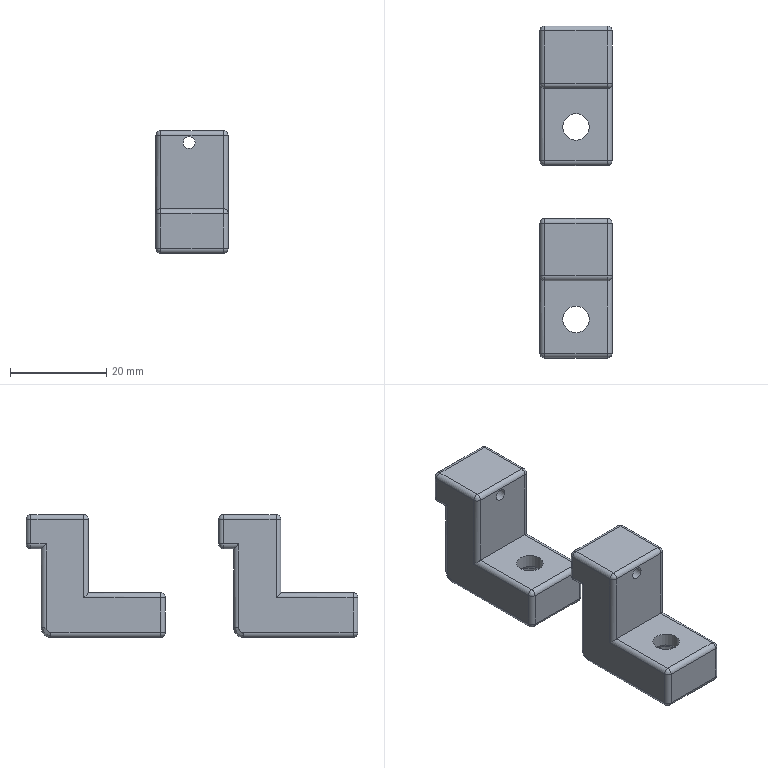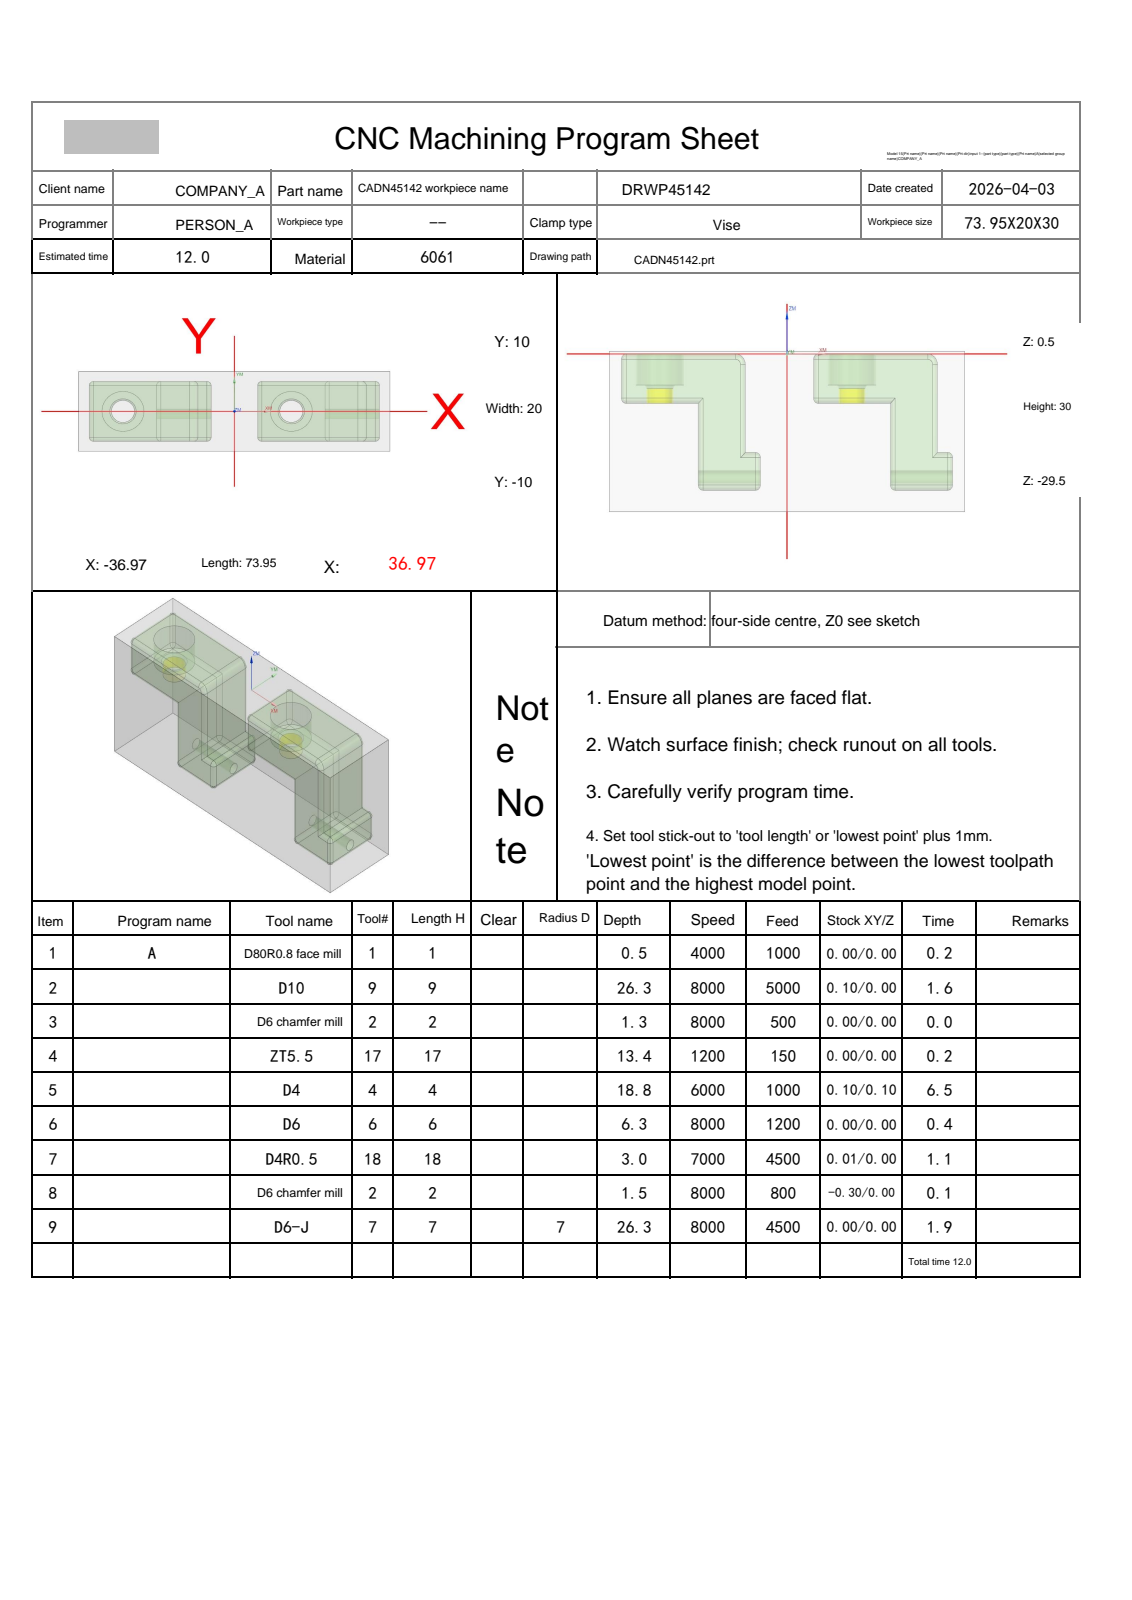NC program | NX | posted by the shop | part box 15 x 68.95 x 25.5 mm
Lines 3215 to 4664 of 6074:
N6 T06 M06
(D6  D=6. R=0. H=06 ce=0.10 di=0.00)
G00 G90 G54 X-26.475 Y0.0 M03 S8000
G43 H06 Z20.
M08
Z.5
G03 X-25.525 Y.95 I0.0 J.95 F1200.
X-26.475 Y1.9 I-.95 J0.0
X-26.475 Y1.9 Z0.0 I0.0 J-1.9
X-26.475 Y1.9 Z-.5 I0.0 J-1.9
X-26.475 Y1.9 Z-1. I0.0 J-1.9
X-26.475 Y1.9 Z-1.5 I0.0 J-1.9
X-26.475 Y1.9 Z-2. I0.0 J-1.9
X-26.475 Y1.9 Z-2.5 I0.0 J-1.9
X-26.475 Y1.9 Z-3. I0.0 J-1.9
X-26.475 Y1.9 Z-3.5 I0.0 J-1.9
X-26.475 Y1.9 Z-4. I0.0 J-1.9
X-26.475 Y1.9 Z-4.5 I0.0 J-1.9
X-26.475 Y1.9 Z-5. I0.0 J-1.9
X-26.475 Y1.9 Z-5.5 I0.0 J-1.9
X-25.358 Y-1.537 Z-5.8 I0.0 J-1.9
X-24.575 Y0.0 I-1.117 J1.537
X-26.475 Y1.9 I-1.9 J0.0
X-28.375 Y0.0 I0.0 J-1.9
X-26.475 Y-1.9 I1.9 J0.0
X-25.358 Y-1.537 I0.0 J1.9
X-24.966 Y-.769 I-.558 J.769
X-25.916 Y.181 I-.95 J0.0
X-26.475 Y0.0 I0.0 J-.95
G00 Z20.
X13.525
Z.5
G03 X14.475 Y.95 I0.0 J.95
X13.525 Y1.9 I-.95 J0.0
X13.525 Y1.9 Z0.0 I0.0 J-1.9
X13.525 Y1.9 Z-.5 I0.0 J-1.9
X13.525 Y1.9 Z-1. I0.0 J-1.9
X13.525 Y1.9 Z-1.5 I0.0 J-1.9
X13.525 Y1.9 Z-2. I0.0 J-1.9
X13.525 Y1.9 Z-2.5 I0.0 J-1.9
X13.525 Y1.9 Z-3. I0.0 J-1.9
X13.525 Y1.9 Z-3.5 I0.0 J-1.9
X13.525 Y1.9 Z-4. I0.0 J-1.9
X13.525 Y1.9 Z-4.5 I0.0 J-1.9
X13.525 Y1.9 Z-5. I0.0 J-1.9
X13.525 Y1.9 Z-5.5 I0.0 J-1.9
X14.642 Y-1.537 Z-5.8 I0.0 J-1.9
X15.425 Y0.0 I-1.117 J1.537
X13.525 Y1.9 I-1.9 J0.0
X11.625 Y0.0 I0.0 J-1.9
X13.525 Y-1.9 I1.9 J0.0
X14.642 Y-1.537 I0.0 J1.9
X15.034 Y-.769 I-.558 J.769
X14.084 Y.181 I-.95 J0.0
X13.525 Y0.0 I0.0 J-.95
G00 Z20.
G00 G90 X-26.475 Y0.0 M03 S8000
Z20.
Z0.0
G41 D06
G01 X-26.279 Y.039 F500.
G03 X-25.485 Y1.01 I-.196 J.97
X-26.475 Y2. I-.99 J0.0
X-26.475 Y2. Z-5. I0.0 J-2.
X-28.163 Y1.071 Z-5.8 I0.0 J-2.
X-28.475 Y0.0 I1.689 J-1.072
X-26.475 Y-2. I2. J0.0
X-24.475 Y0.0 I0.0 J2.
X-26.475 Y2. I-2. J0.0
X-28.163 Y1.071 I0.0 J-2.
X-28.318 Y.541 I.836 J-.53
X-27.328 Y-.449 I.99 J0.0
X-26.613 Y-.145 I0.0 J.99
G01 G40 X-26.475 Y0.0
G00 Z20.
X13.525
Z0.0
G41 D06
G01 X13.721 Y.039
G03 X14.515 Y1.01 I-.196 J.97
X13.525 Y2. I-.99 J0.0
X13.525 Y2. Z-5. I0.0 J-2.
X11.837 Y1.071 Z-5.8 I0.0 J-2.
X11.525 Y0.0 I1.689 J-1.072
X13.525 Y-2. I2. J0.0
X15.525 Y0.0 I0.0 J2.
X13.525 Y2. I-2. J0.0
X11.837 Y1.071 I0.0 J-2.
X11.682 Y.541 I.836 J-.53
X12.672 Y-.449 I.99 J0.0
X13.387 Y-.145 I0.0 J.99
G01 G40 X13.525 Y0.0
G00 Z20.
G91 G28 Z0.0
M05
M09
G91 G28 Z0.0
M01
N7 T18 M06
(D4R0.5  D=4. R=0.5 H=18 ce=0.01 di=0.00)
G00 G90 G54 X33.75 Y-7.915 M03 S7000
G43 H18 Z10.5
M08
Z.488
G01 Z-.012 F4500.
X30.426 Y-8.129
X29.326 Y-8.2
X6.525
G02 X4.825 Y-6.5 I0.0 J1.7
G01 Y6.5
G02 X6.525 Y8.2 I1.7 J0.0
G01 X29.325
X30.425 Y8.129
Y8.224 Z-.021
Y8.27 Z-.03
X29.325 Y8.309
X6.525
G03 X4.716 Y6.5 I0.0 J-1.809
G01 Y-6.5
G03 X6.525 Y-8.309 I1.809 J0.0
G01 X29.326
X30.426 Y-8.271
Y-8.345 Z-.042
X30.427 Y-8.391 Z-.054
X29.326 Y-8.408
X6.525
G02 X4.617 Y-6.5 I0.0 J1.909
G01 Y6.5
G02 X6.525 Y8.408 I1.909 J0.0
G01 X29.325
X30.425 Y8.387
X30.325 Y8.479 Z-.084
X29.325 Y8.504
X6.525
G03 X4.521 Y6.5 I0.0 J-2.004
G01 Y-6.5
G03 X6.525 Y-8.504 I2.004 J0.0
G01 X29.326
X30.426 Y-8.48
Y-8.528 Z-.102
Y-8.576 Z-.119
X29.326 Y-8.597
X6.525
G02 X4.429 Y-6.5 I0.0 J2.097
G01 Y6.5
G02 X6.525 Y8.597 I2.097 J0.0
G01 X29.325
X30.426 Y8.573
Y8.621 Z-.14
Y8.667 Z-.161
X29.325 Y8.687
X6.525
G03 X4.338 Y6.5 I0.0 J-2.187
G01 Y-6.5
G03 X6.525 Y-8.687 I2.187 J0.0
G01 X29.326
X30.437 Y-8.667
X30.433 Y-8.713 Z-.185
X30.429 Y-8.762 Z-.209
X29.326 Y-8.774
X6.525
G02 X4.251 Y-6.5 I0.0 J2.274
G01 Y6.5
G02 X6.525 Y8.774 I2.274 J0.0
G01 X29.325
X30.426 Y8.761
Y8.802 Z-.236
Y8.838 Z-.263
X29.325 Y8.858
X6.525
G03 X4.167 Y6.5 I0.0 J-2.359
G01 Y-6.5
G03 X6.525 Y-8.858 I2.359 J0.0
G01 X29.326
X30.426 Y-8.846
Y-8.885 Z-.293
X30.427 Y-8.918 Z-.322
X29.326 Y-8.939
X6.525
G02 X4.087 Y-6.5 I0.0 J2.439
G01 Y6.5
G02 X6.525 Y8.939 I2.439 J0.0
G01 X29.325
X30.421 Y8.916
Y8.952 Z-.354
Y8.989 Z-.386
X29.325 Y9.014
X6.525
G03 X4.011 Y6.5 I0.0 J-2.515
G01 Y-6.5
G03 X6.525 Y-9.014 I2.515 J0.0
G01 X29.326
X30.427 Y-8.99
Y-9.026 Z-.421
X30.426 Y-9.063 Z-.455
G03 X30.169 Y-9.061 I-.257 J-13.991
X29.326 Y-9.086 I0.0 J-13.993
G01 X6.525
G02 X3.939 Y-6.5 I0.0 J2.586
G01 Y6.5
G02 X6.525 Y9.086 I2.586 J0.0
G01 X29.325
G03 X30.178 Y9.059 I.853 J13.444
X30.421 Y9.061 I0.0 J13.471
G01 X30.424 Y9.099 Z-.492
X30.426 Y9.13 Z-.529
G02 X30.148 Y9.127 I-.279 J12.986
X29.325 Y9.153 I0.0 J12.989
G01 X6.525
G03 X3.872 Y6.5 I0.0 J-2.653
G01 Y-6.5
G03 X6.525 Y-9.153 I2.653 J0.0
G01 X29.326
G02 X30.192 Y-9.129 I.866 J-15.495
X30.426 Y-9.131 I0.0 J-15.52
G01 X30.427 Y-9.165 Z-.568
Y-9.196 Z-.607
G03 X29.326 Y-9.215 I1.173 J-101.223
G01 X6.525
G02 X3.81 Y-6.5 I0.0 J2.715
G01 Y6.5
G02 X6.525 Y9.215 I2.715 J0.0
G01 X29.325
X30.426 Y9.2
Y9.23 Z-.648
Y9.262 Z-.689
X29.325 Y9.272
X6.525
G03 X3.753 Y6.5 I0.0 J-2.772
G01 Y-6.5
G03 X6.525 Y-9.272 I2.772 J0.0
G01 X29.326
G02 X30.246 Y-9.258 I.92 J-31.243
G01 X30.427 Y-9.259
X30.426 Y-9.291 Z-.732
Y-9.316 Z-.775
X29.326 Y-9.323
X6.525
G02 X3.702 Y-6.5 I0.0 J2.823
G01 Y6.5
G02 X6.525 Y9.323 I2.823 J0.0
G01 X29.325
X30.425 Y9.316
X30.426 Y9.337 Z-.82
Y9.358 Z-.864
X29.325 Y9.368
X6.525
G03 X3.657 Y6.5 I0.0 J-2.869
G01 Y-6.5
G03 X6.525 Y-9.368 I2.869 J0.0
G01 X29.326
X30.426 Y-9.358
Y-9.376 Z-.91
Y-9.397 Z-.956
X30.392
X29.326 Y-9.408
X6.525
G02 X3.617 Y-6.5 I0.0 J2.908
G01 Y6.5
G02 X6.525 Y9.408 I2.908 J0.0
G01 X29.325
X30.392 Y9.396
X30.426 Y9.397
Y9.414 Z-1.003
Y9.428 Z-1.051
X30.22 Y9.427
G02 X29.325 Y9.441 I0.0 J29.627
G01 X6.525
G03 X3.584 Y6.5 I0.0 J-2.941
G01 Y-6.5
G03 X6.525 Y-9.441 I2.941 J0.0
G01 X29.326
G02 X30.193 Y-9.427 I.867 J-27.33
G01 X30.427 Y-9.428
X30.424 Y-9.446 Z-1.099
X30.422 Y-9.458 Z-1.147
X29.326 Y-9.468
X6.525
G02 X3.557 Y-6.5 I0.0 J2.968
G01 Y6.5
G02 X6.525 Y9.468 I2.968 J0.0
G01 X29.325
X30.422 Y9.458
Y9.462 Z-1.191
Y9.477 Z-1.235
X29.325 Y9.486
X6.525
G03 X3.539 Y6.5 I0.0 J-2.986
G01 Y-6.5
G03 X6.525 Y-9.486 I2.986 J0.0
G01 X29.326
X30.422 Y-9.477
Y-9.484 Z-1.279
Y-9.49 Z-1.323
G03 X30.133 Y-9.488 I-.289 J-29.016
X29.326 Y-9.499 I0.0 J-29.017
G01 X6.525
G02 X3.526 Y-6.5 I0.0 J3.
G01 Y6.5
G02 X6.525 Y9.499 I3. J0.0
G01 X29.325
G03 X30.137 Y9.488 I.811 J29.996
X30.422 Y9.49 I0.0 J30.007
G01 Y9.494 Z-1.368
Y9.5 Z-1.412
X29.325 Y9.507
X6.525
G03 X3.518 Y6.5 I0.0 J-3.007
G01 Y-6.5
G03 X6.525 Y-9.507 I3.007 J0.0
G01 X29.326
X30.422 Y-9.5
Y-9.51 Z-1.5
X29.326
X6.525
X6.404 Y-9.507
G02 X3.517 Y-6.615 I.121 J3.008
G01 X3.516 Y-6.561
Y6.5
X3.517 Y6.615
G02 X6.404 Y9.507 I3.008 J-.115
G01 X6.525 Y9.51
X29.325
X30.422
G00 Z10.5
X-6.38 Y-8.25
Z.488
G01 Z-.012
X-9.574 Y-8.129
X-10.674 Y-8.2
X-33.475
G02 X-35.175 Y-6.5 I0.0 J1.7
G01 Y6.5
G02 X-33.475 Y8.2 I1.7 J0.0
G01 X-10.675
X-9.575 Y8.129
Y8.224 Z-.021
Y8.27 Z-.03
X-10.675 Y8.309
X-33.475
G03 X-35.284 Y6.5 I0.0 J-1.809
G01 Y-6.5
G03 X-33.475 Y-8.309 I1.809 J0.0
G01 X-10.674
X-9.574 Y-8.27
Y-8.345 Z-.042
Y-8.385 Z-.054
X-9.631 Y-8.375
X-10.659 Y-8.402
X-10.674 Y-8.408
X-33.475
G02 X-35.383 Y-6.5 I0.0 J1.909
G01 Y6.5
G02 X-33.475 Y8.408 I1.909 J0.0
G01 X-10.675
X-9.575 Y8.386
X-9.574 Y8.438 Z-.069
Y8.479 Z-.084
X-10.675 Y8.504
X-33.475
G03 X-35.479 Y6.5 I0.0 J-2.004
G01 Y-6.5
G03 X-33.475 Y-8.504 I2.004 J0.0
G01 X-10.674
X-9.574 Y-8.478
Y-8.529 Z-.102
X-9.573 Y-8.571 Z-.119
X-10.674 Y-8.597
X-33.475
G02 X-35.571 Y-6.5 I0.0 J2.097
G01 Y6.5
G02 X-33.475 Y8.597 I2.097 J0.0
G01 X-10.675
X-9.574 Y8.573
Y8.62 Z-.14
Y8.667 Z-.161
X-10.675 Y8.687
X-33.475
G03 X-35.662 Y6.5 I0.0 J-2.187
G01 Y-6.5
G03 X-33.475 Y-8.687 I2.187 J0.0
G01 X-10.674
X-9.57 Y-8.667
X-9.569 Y-8.713 Z-.185
X-9.567 Y-8.763 Z-.209
X-10.674 Y-8.774
X-33.475
G02 X-35.749 Y-6.5 I0.0 J2.274
G01 Y6.5
G02 X-33.475 Y8.774 I2.274 J0.0
G01 X-10.675
X-9.574 Y8.761
Y8.802 Z-.236
Y8.838 Z-.263
X-10.659 Y8.855
X-10.675 Y8.858
X-33.475
G03 X-35.833 Y6.5 I0.0 J-2.359
G01 Y-6.5
G03 X-33.475 Y-8.858 I2.359 J0.0
G01 X-10.674
X-9.574 Y-8.845
Y-8.88 Z-.293
Y-8.918 Z-.322
X-10.674 Y-8.939
X-33.475
G02 X-35.913 Y-6.5 I0.0 J2.439
G01 Y6.5
G02 X-33.475 Y8.939 I2.439 J0.0
G01 X-10.675
X-9.574 Y8.916
Y8.952 Z-.354
Y8.989 Z-.386
X-10.675 Y9.014
X-33.475
G03 X-35.989 Y6.5 I0.0 J-2.515
G01 Y-6.5
G03 X-33.475 Y-9.014 I2.515 J0.0
G01 X-10.674
X-9.574 Y-8.99
Y-9.029 Z-.421
X-9.575 Y-9.063 Z-.455
X-9.608 Y-9.061
X-10.659 Y-9.081
X-10.674 Y-9.086
X-33.475
G02 X-36.061 Y-6.5 I0.0 J2.586
G01 Y6.5
G02 X-33.475 Y9.086 I2.586 J0.0
G01 X-10.675
X-10.659 Y9.081
X-9.621 Y9.063
X-9.574 Y9.064
Y9.099 Z-.492
X-9.575 Y9.132 Z-.529
G02 X-9.872 Y9.128 I-.297 J13.112
X-10.675 Y9.153 I0.0 J13.115
G01 X-33.475
G03 X-36.128 Y6.5 I0.0 J-2.653
G01 Y-6.5
G03 X-33.475 Y-9.153 I2.653 J0.0
G01 X-10.674
X-10.659 Y-9.15
X-9.573 Y-9.129
Y-9.165 Z-.568
Y-9.198 Z-.607
X-10.659 Y-9.21
X-10.674 Y-9.215
X-33.475
G02 X-36.19 Y-6.5 I0.0 J2.715
G01 Y6.5
G02 X-33.475 Y9.215 I2.715 J0.0
G01 X-10.675
X-9.575 Y9.2
Y9.23 Z-.648
Y9.263 Z-.689
X-10.659 Y9.266
X-10.675 Y9.272
X-33.475
G03 X-36.247 Y6.5 I0.0 J-2.772
G01 Y-6.5
G03 X-33.475 Y-9.272 I2.772 J0.0
G01 X-10.674
X-10.659 Y-9.266
X-9.574 Y-9.261
Y-9.291 Z-.732
Y-9.316 Z-.775
X-10.674 Y-9.323
X-33.475
G02 X-36.298 Y-6.5 I0.0 J2.823
G01 Y6.5
G02 X-33.475 Y9.323 I2.823 J0.0
G01 X-10.675
X-9.575 Y9.316
Y9.337 Z-.82
X-9.574 Y9.358 Z-.864
X-10.675 Y9.368
X-33.475
G03 X-36.343 Y6.5 I0.0 J-2.869
G01 Y-6.5
G03 X-33.475 Y-9.368 I2.869 J0.0
G01 X-10.674
X-9.574 Y-9.358
Y-9.376 Z-.91
Y-9.396 Z-.956
X-10.674 Y-9.408
X-33.475
G02 X-36.383 Y-6.5 I0.0 J2.908
G01 Y6.5
G02 X-33.475 Y9.408 I2.908 J0.0
G01 X-10.675
X-9.574 Y9.396
Y9.413 Z-1.003
Y9.428 Z-1.051
X-10.659 Y9.438
X-10.675 Y9.441
X-33.475
G03 X-36.416 Y6.5 I0.0 J-2.941
G01 Y-6.5
G03 X-33.475 Y-9.441 I2.941 J0.0
G01 X-10.674
X-10.659 Y-9.438
X-9.573 Y-9.428
X-9.572 Y-9.446 Z-1.099
X-9.571 Y-9.458 Z-1.147
X-10.674 Y-9.468
X-33.475
G02 X-36.443 Y-6.5 I0.0 J2.968
G01 Y6.5
G02 X-33.475 Y9.468 I2.968 J0.0
G01 X-10.675
X-9.571 Y9.458
Y9.462 Z-1.191
Y9.477 Z-1.235
X-10.675 Y9.486
X-33.475
G03 X-36.461 Y6.5 I0.0 J-2.986
G01 Y-6.5
G03 X-33.475 Y-9.486 I2.986 J0.0
G01 X-10.674
X-9.571 Y-9.477
Y-9.484 Z-1.279
Y-9.49 Z-1.323
X-10.659 Y-9.498
X-10.674 Y-9.499
X-33.475
G02 X-36.474 Y-6.5 I0.0 J3.
G01 Y6.5
G02 X-33.475 Y9.499 I3. J0.0
G01 X-10.675
X-10.659 Y9.498
X-9.571 Y9.49
Y9.494 Z-1.368
Y9.5 Z-1.412
X-10.659 Y9.504
X-10.675 Y9.507
X-33.475
G03 X-36.482 Y6.5 I0.0 J-3.007
G01 Y-6.5
G03 X-33.475 Y-9.507 I3.007 J0.0
G01 X-10.674
X-10.659 Y-9.504
X-9.571 Y-9.5
Y-9.51 Z-1.5
X-33.475
X-33.59 Y-9.508
G02 X-36.483 Y-6.615 I.115 J3.008
G01 X-36.484 Y-6.5
Y6.5
X-36.483 Y6.615
G02 X-33.475 Y9.51 I3.008 J-.115
G01 X-10.675
X-9.571
G00 Z10.5
G00 G90 X27.61 Y8.973 M03 S7000
Z10.5
Z.491
G01 Z-.009 F4500.
Y8.949
G03 X28.214 Y8.173 I.8 J0.0
X28.788 Y8.102 I.575 J2.272
X29.084 Y8.121 I0.0 J2.343
G02 X29.304 Y8.134 I.22 J-1.733
X31.047 Y6.5 I0.0 J-1.746
G01 Y-6.48
G02 X29.334 Y-8.166 I-1.812 J.127
G01 X29.263 Y-8.116
X28.214 Y-8.173
Y-8.223 Z-.015
Y-8.262 Z-.021
X29.263 Y-8.222
X29.334 Y-8.252
G03 X31.162 Y-6.5 I-.057 J1.889
G01 Y6.5
G03 X29.274 Y8.254 I-1.888 J-.139
G01 X29.192 Y8.252
X29.051 Y8.222
X28.214 Y8.262
Y8.306 Z-.03
Y8.345 Z-.038
X29.562 Y8.326
X29.617 Y8.316
G02 X31.269 Y6.5 I-.321 J-1.951
G01 Y-6.5
G02 X29.334 Y-8.342 I-1.973 J.136
G01 X28.214 Y-8.345
Y-8.386 Z-.048
Y-8.424 Z-.058
X29.617 Y-8.381
X29.735 Y-8.36
G03 X31.372 Y-6.5 I-.344 J1.954
G01 Y6.5
G03 X29.461 Y8.386 I-1.971 J-.086
G01 X28.214 Y8.424
Y8.464 Z-.07
Y8.5 Z-.083
G02 X28.757 Y8.531 I.544 J-4.85
X30.067 Y8.352 I0.0 J-4.881
X31.472 Y6.502 I-.515 J-1.85
G01 X31.473 Y-6.502
G02 X30.068 Y-8.352 I-1.92 J0.0
X28.758 Y-8.531 I-1.31 J4.705
X28.214 Y-8.5 I0.0 J4.884
G01 Y-8.539 Z-.097
Y-8.575 Z-.111
G03 X28.762 Y-8.604 I.548 J5.132
X29.966 Y-8.462 I0.0 J5.161
X31.571 Y-6.5 I-.489 J2.038
G01 Y6.5
G03 X29.966 Y8.462 I-2.095 J-.076
X28.762 Y8.604 I-1.204 J-5.014
X28.214 Y8.575 I0.0 J-5.157
G01 Y8.613 Z-.127
Y8.648 Z-.143
X29.617 Y8.623
X29.901 Y8.568
G02 X31.668 Y6.5 I-.446 J-2.17
G01 Y-6.5
G02 X29.901 Y-8.568 I-2.213 J.102
G01 X29.617 Y-8.623
X28.214 Y-8.648
Y-8.685 Z-.16
Y-8.719 Z-.178
X29.617 Y-8.692
X29.833 Y-8.659
G03 X31.763 Y-6.5 I-.351 J2.256
G01 Y6.5
G03 X29.833 Y8.659 I-2.281 J-.098
G01 X29.617 Y8.692
X28.214 Y8.719
Y8.755 Z-.198
Y8.788 Z-.218
G02 X28.68 Y8.8 I.466 J-9.521
X29.773 Y8.737 I0.0 J-9.532
X31.856 Y6.5 I-.27 J-2.339
G01 Y-6.5
G02 X29.773 Y-8.737 I-2.353 J.103
X28.68 Y-8.8 I-1.093 J9.48
X28.214 Y-8.788 I0.0 J9.543
G01 Y-8.823 Z-.239
Y-8.855 Z-.261
G03 X28.678 Y-8.866 I.464 J9.729
X29.799 Y-8.801 I0.0 J9.741
X31.948 Y-6.5 I-.28 J2.414
G01 X31.947 Y6.5
G03 X29.799 Y8.801 I-2.428 J-.113
X28.678 Y8.866 I-1.121 J-9.667
X28.214 Y8.855 I0.0 J-9.732
G01 Y8.888 Z-.284
Y8.92 Z-.307
G02 X28.763 Y8.939 I.549 J-7.787
X29.888 Y8.858 I0.0 J-7.806
X31.915 Y7.197 I-.366 J-2.514
G01 X32.021 Y6.632
X32.037 Y6.5
Y-6.5
G02 X30.868 Y-8.489 I-2.443 J.098
X29.685 Y-8.89 I-1.484 J2.429
X28.749 Y-8.934 I-.936 J9.962
X28.214 Y-8.92 I0.0 J10.006
G01 Y-8.952 Z-.333
Y-8.982 Z-.358
G03 X28.743 Y-9. I.529 J7.765
X30.046 Y-8.89 I0.0 J7.784
X32.124 Y-6.5 I-.456 J2.495
G01 Y6.5
G03 X30.046 Y8.89 I-2.535 J-.105
X28.743 Y9. I-1.303 J-7.673
X28.214 Y8.982 I0.0 J-7.783
G01 Y9.013 Z-.384
Y9.042 Z-.411
G02 X28.757 Y9.052 I.543 J-14.026
X29.537 Y9.03 I0.0 J-14.036
X31.03 Y8.558 I-.175 J-3.148
X32.209 Y6.5 I-1.325 J-2.126
G01 Y-6.5
G02 X30.751 Y-8.717 I-2.534 J.078
X29.334 Y-9.04 I-1.462 J3.139
G01 X28.228
X28.214 Y-9.042
Y-9.071 Z-.44
Y-9.098 Z-.468
G03 X28.709 Y-9.107 I.495 J14.3
X29.617 Y-9.078 I0.0 J14.309
X31.034 Y-8.637 I-.217 J3.195
X32.292 Y-6.5 I-1.314 J2.212
G01 Y6.5
G03 X31.919 Y7.761 I-2.546 J-.068
X29.798 Y9.058 I-2.405 J-1.551
X28.735 Y9.111 I-1.063 J-10.631
X28.214 Y9.098 I0.0 J-10.684
G01 Y9.126 Z-.498
Y9.153 Z-.528
G02 X28.758 Y9.168 I.544 J-9.529
X29.901 Y9.099 I0.0 J-9.545
X31.884 Y7.962 I-.397 J-2.992
X32.372 Y6.5 I-2.25 J-1.564
G01 X32.373 Y-6.5
G02 X31.2 Y-8.608 I-2.607 J.07
X29.617 Y-9.132 I-1.784 J2.734
X28.746 Y-9.165 I-.871 J11.643
X28.214 Y-9.153 I0.0 J11.676
G01 Y-9.179 Z-.56
Y-9.203 Z-.591
X28.228 Y-9.202
X29.334
X29.347
G03 X31.318 Y-8.61 I0.0 J3.578
X32.451 Y-6.5 I-1.534 J2.183
G01 X32.45 Y6.5
G03 X31.318 Y8.61 I-2.668 J-.073
X29.346 Y9.202 I-1.971 J-2.986
G01 X29.334
X28.227
X28.214 Y9.203
Y9.228 Z-.625
Y9.251 Z-.658
X29.334
X29.338
G02 X31.034 Y8.849 I0.0 J-3.776
X32.526 Y6.5 I-1.207 J-2.414
G01 Y-6.5
G02 X31.034 Y-8.849 I-2.698 J.065
X29.339 Y-9.251 I-1.696 J3.376
G01 X29.334
X28.214
Y-9.274 Z-.692
Y-9.295 Z-.727
X29.334
X29.346
G03 X31.034 Y-8.915 I0.0 J3.936
X32.598 Y-6.5 I-1.184 J2.481
G01 Y6.5
G03 X31.318 Y8.753 I-2.716 J-.054
X29.617 Y9.281 I-1.873 J-3.031
X28.6 Y9.298 I-1.017 J-30.065
X28.214 Y9.295 I0.0 J-30.082
G01 Y9.316 Z-.763
Y9.336 Z-.799
G02 X28.761 Y9.349 I.547 J-11.927
X29.901 Y9.294 I0.0 J-11.94
X31.601 Y8.621 I-.348 J-3.364
X32.668 Y6.5 I-1.652 J-2.16
G01 Y-6.5
G02 X31.318 Y-8.817 I-2.74 J.045
X29.901 Y-9.294 I-1.801 J3.002
X28.761 Y-9.349 I-1.139 J11.897
X28.214 Y-9.336 I0.0 J11.951
G01 Y-9.355 Z-.837
Y-9.373 Z-.874
X28.228 Y-9.372
X29.334
G03 X30.775 Y-9.131 I-.021 J4.565
X31.698 Y-8.608 I-.9 J2.661
G01 X31.884 Y-8.456
G03 X32.735 Y-6.5 I-1.936 J2.005
G01 X32.734 Y6.5
G03 X32.411 Y7.761 I-2.856 J-.06
X30.751 Y9.14 I-2.605 J-1.447
X29.334 Y9.372 I-1.437 J-4.341
G01 X28.227
X28.214 Y9.373
Y9.39 Z-.913
Y9.406 Z-.951
X28.227 Y9.403
X29.334
X29.372
G02 X30.467 Y9.264 I0.0 J-4.385
G01 X30.751 Y9.187
G02 X31.884 Y8.525 I-1.007 J-3.027
X32.798 Y6.5 I-1.859 J-2.058
G01 Y-6.5
G02 X31.884 Y-8.526 I-2.773 J.032
X30.751 Y-9.187 I-2.14 J2.365
G01 X30.467 Y-9.264
G02 X29.372 Y-9.403 I-1.095 J4.246
G01 X29.334
X28.228
X28.214 Y-9.406
Y-9.421 Z-.991
Y-9.435 Z-1.031
G03 X28.727 Y-9.443 I.513 J16.619
X29.901 Y-9.401 I0.0 J16.627
X31.488 Y-8.89 I-.312 J3.69
X32.859 Y-6.5 I-1.479 J2.437
G01 Y6.5
G03 X31.487 Y8.89 I-2.85 J-.047
X29.901 Y9.401 I-1.899 J-3.179
X28.727 Y9.443 I-1.174 J-16.57
X28.214 Y9.435 I0.0 J-16.612
G01 X28.216 Y9.448 Z-1.072
X28.218 Y9.459 Z-1.114
G02 X28.771 Y9.47 I.552 J-14.81
X29.901 Y9.426 I0.0 J-14.821
X31.601 Y8.871 I-.243 J-3.624
X32.916 Y6.5 I-1.559 J-2.414
G01 Y-6.5
G02 X31.601 Y-8.871 I-2.873 J.043
X29.901 Y-9.426 I-1.943 J3.068
X28.771 Y-9.47 I-1.13 J14.793
X28.218 Y-9.459 I0.0 J14.836
G01 Y-9.47 Z-1.156
Y-9.479 Z-1.198
X29.334 Y-9.477
X29.359
G03 X30.467 Y-9.371 I0.0 J5.888
X31.884 Y-8.72 I-.666 J3.313
X32.97 Y-6.5 I-1.806 J2.259
G01 Y6.5
G03 X32.878 Y7.197 I-4.117 J-.185
X31.034 Y9.202 I-2.865 J-.784
X29.617 Y9.471 I-1.51 J-4.089
G01 X28.218 Y9.479
Y9.487 Z-1.241
Y9.494 Z-1.284
G02 X29.617 Y9.486 I-.232 J-162.856
X31.203 Y9.172 I-.032 J-4.322
X32.719 Y7.761 I-1.193 J-2.802
X33.02 Y6.5 I-2.787 J-1.332
G01 Y-6.5
G02 X31.884 Y-8.775 I-2.93 J.042
X30.196 Y-9.441 I-2.097 J2.84
X29.363 Y-9.49 I-.833 J7.145
G01 X28.236
X28.218 Y-9.494
Y-9.504 Z-1.373
X28.236 Y-9.499
G03 X28.757 Y-9.502 I.521 J41.295
X29.901 Y-9.486 I0.0 J41.298
X31.318 Y-9.155 I-.181 J3.972
X33.067 Y-6.5 I-1.21 J2.701
G01 Y6.5
G03 X31.318 Y9.155 I-2.959 J-.046
X29.901 Y9.486 I-1.598 J-3.64
X28.755 Y9.502 I-1.146 J-41.506
X28.236 Y9.499 I0.0 J-41.522
G01 X28.218 Y9.504
Y9.509 Z-1.463
G02 X28.761 Y9.515 I.543 J-27.928
X30.09 Y9.483 I0.0 J-27.934
X32.168 Y8.632 I-.16 J-3.351
X33.11 Y6.5 I-2.058 J-2.184
G01 X33.111 Y-6.5
G02 X32.168 Y-8.633 I-3.001 J.052
X30.075 Y-9.483 I-2.237 J2.503
X28.697 Y-9.513 I-1.378 J32.018
X28.218 Y-9.509 I0.0 J32.048
G01 Y-9.51 Z-1.555
X29.617
X29.999 Y-9.498
G03 X31.312 Y-9.215 I-.119 J3.744
X33.018 Y-7.349 I-1.138 J2.752
X33.15 Y-6.5 I-3.615 J1.
G01 Y6.5
G03 X33.018 Y7.349 I-3.761 J-.152
X31.312 Y9.215 I-2.844 J-.886
X30.001 Y9.498 I-1.431 J-3.46
G01 X29.617 Y9.51
X28.218
Z-1.648
X29.617
X29.901 Y9.508
X29.923
G02 X31.318 Y9.241 I0.0 J-3.769
X33.186 Y6.5 I-1.122 J-2.772
G01 Y-6.5
G02 X31.318 Y-9.241 I-2.991 J.031
X29.922 Y-9.509 I-1.395 J3.505
G01 X29.901
X29.617 Y-9.51
X28.218
Z-1.743
X29.901
X30.184 Y-9.502
G03 X31.884 Y-8.967 I-.109 J3.317
X33.218 Y-6.5 I-1.662 J2.493
G01 Y6.5
G03 X31.884 Y8.967 I-2.996 J-.026
X30.184 Y9.502 I-1.81 J-2.783
G01 X29.901 Y9.51
X28.218
Z-1.839
X29.901
X30.184 Y9.505
G02 X32.363 Y8.608 I-.043 J-3.2
X33.246 Y6.5 I-2.149 J-2.139
G01 X33.247 Y-6.5
G02 X31.561 Y-9.172 I-2.999 J.023
G01 X31.318 Y-9.284
X31.034 Y-9.376
G02 X30.184 Y-9.505 I-.894 J3.014
G01 X29.901 Y-9.51
X28.218
Z-1.936
X30.184 Y-9.509
X30.361 Y-9.5
G03 X32.734 Y-8.201 I-.147 J3.085
X33.271 Y-6.5 I-2.563 J1.745
G01 Y6.5
G03 X32.734 Y8.2 I-3.102 J-.044
X30.361 Y9.5 I-2.52 J-1.786
G01 X30.184 Y9.509
X28.218 Y9.51
Z-2.034
X30.184
X30.361 Y9.503
G02 X32.858 Y8.043 I-.113 J-3.058
X33.292 Y6.5 I-2.658 J-1.58
G01 Y-6.5
G02 X30.751 Y-9.46 I-3.019 J.02
X30.184 Y-9.51 I-.629 J3.932
G01 X28.218
Z-2.133
X30.184
X30.361 Y-9.505
G03 X31.884 Y-9.051 I-.125 J3.198
X33.309 Y-6.5 I-1.617 J2.576
G01 X33.308 Y6.5
G03 X32.734 Y8.258 I-3.086 J-.035
X30.343 Y9.504 I-2.459 J-1.802
G01 X30.184 Y9.51
X28.218
Z-2.224
X30.184
X30.343 Y9.506
G02 X32.734 Y8.275 I-.055 J-3.045
X33.31 Y6.632 I-2.44 J-1.778
G01 X33.313 Y6.566
X33.32 Y6.5
X33.321 Y-6.5
X33.315 Y-6.516
X33.311 Y-6.632
G02 X31.671 Y-9.172 I-2.984 J.127
G01 X31.601 Y-9.208
G02 X30.343 Y-9.506 I-1.319 J2.763
G01 X30.184 Y-9.51
X28.218
Z-2.316
X30.361 Y-9.509
X30.467 Y-9.503
G03 X33.301 Y-6.866 I-.158 J3.011
G01 X33.329 Y-6.5
Y6.5
X33.322 Y6.566
X33.301 Y6.863
G03 X30.467 Y9.503 I-2.992 J-.371
G01 X30.361 Y9.509
X28.218 Y9.51
Z-2.408
X30.343
G02 X33.334 Y6.5 I-.032 J-3.022
G01 Y-6.5
G02 X30.343 Y-9.51 I-3.022 J.012
G01 X28.218
Z-2.5
X30.343
G03 X33.336 Y-6.5 I-.019 J3.011
G01 Y-.141
X33.335 Y6.49
Y6.498
G03 X30.343 Y9.51 I-3.011 J0.0
G01 X28.218
G00 Z10.5
X-12.39 Y8.973
Z.491
G01 Z-.009
Y8.949
G03 X-11.786 Y8.173 I.8 J0.0
X-11.212 Y8.102 I.575 J2.272
X-10.916 Y8.121 I0.0 J2.343
G02 X-10.696 Y8.134 I.22 J-1.733
X-8.953 Y6.5 I0.0 J-1.746
G01 Y-6.48
G02 X-10.666 Y-8.166 I-1.812 J.127
G01 X-10.737 Y-8.116
X-11.786 Y-8.173
Y-8.223 Z-.015
Y-8.262 Z-.021
X-10.737 Y-8.222
X-10.666 Y-8.252
G03 X-8.838 Y-6.5 I-.057 J1.889
G01 Y6.5
G03 X-10.726 Y8.254 I-1.888 J-.139
G01 X-10.808 Y8.252
X-10.949 Y8.222
X-11.786 Y8.262
Y8.306 Z-.03
Y8.345 Z-.038
X-10.438 Y8.326
X-10.383 Y8.316
G02 X-8.731 Y6.5 I-.321 J-1.951
G01 Y-6.5
G02 X-10.666 Y-8.342 I-1.973 J.136
G01 X-11.786 Y-8.345
Y-8.386 Z-.048
Y-8.424 Z-.058
X-10.383 Y-8.381
X-10.265 Y-8.36
G03 X-8.628 Y-6.5 I-.344 J1.954
G01 Y6.5
G03 X-10.539 Y8.386 I-1.971 J-.086
G01 X-11.786 Y8.424
Y8.464 Z-.07
Y8.5 Z-.083
G02 X-11.243 Y8.531 I.544 J-4.85
X-9.933 Y8.352 I0.0 J-4.881
X-8.528 Y6.502 I-.515 J-1.85
G01 X-8.527 Y-6.502
G02 X-9.932 Y-8.352 I-1.92 J0.0
X-11.243 Y-8.531 I-1.31 J4.705
X-11.786 Y-8.5 I0.0 J4.884
G01 Y-8.539 Z-.097
Y-8.575 Z-.111
G03 X-11.238 Y-8.604 I.548 J5.132
X-10.034 Y-8.462 I0.0 J5.161
X-8.429 Y-6.5 I-.489 J2.038
G01 Y6.5
G03 X-10.034 Y8.462 I-2.095 J-.076
X-11.238 Y8.604 I-1.204 J-5.014
X-11.786 Y8.575 I0.0 J-5.157
G01 Y8.613 Z-.127
Y8.648 Z-.143
X-10.383 Y8.623
X-10.099 Y8.568
G02 X-8.332 Y6.5 I-.446 J-2.17
G01 Y-6.5
G02 X-10.099 Y-8.568 I-2.213 J.102
G01 X-10.383 Y-8.623
X-11.786 Y-8.648
Y-8.685 Z-.16
Y-8.719 Z-.178
X-10.383 Y-8.692
X-10.167 Y-8.659
G03 X-8.237 Y-6.5 I-.351 J2.256
G01 Y6.5
G03 X-10.167 Y8.659 I-2.281 J-.098
G01 X-10.383 Y8.692
X-11.786 Y8.719
Y8.755 Z-.198
Y8.788 Z-.218
G02 X-11.32 Y8.8 I.466 J-9.521
X-10.227 Y8.737 I0.0 J-9.532
X-8.144 Y6.5 I-.27 J-2.339
G01 Y-6.5
G02 X-10.227 Y-8.737 I-2.353 J.103
X-11.32 Y-8.8 I-1.093 J9.48
X-11.786 Y-8.788 I0.0 J9.543
G01 Y-8.823 Z-.239
Y-8.855 Z-.261
G03 X-11.322 Y-8.866 I.464 J9.729
X-10.201 Y-8.801 I0.0 J9.741
X-8.052 Y-6.5 I-.28 J2.414
G01 X-8.053 Y6.5
G03 X-10.201 Y8.801 I-2.428 J-.113
X-11.322 Y8.866 I-1.121 J-9.667
X-11.786 Y8.855 I0.0 J-9.732
G01 Y8.888 Z-.284
Y8.92 Z-.307
G02 X-11.237 Y8.939 I.549 J-7.787
X-10.112 Y8.858 I0.0 J-7.806
X-8.085 Y7.197 I-.366 J-2.514
G01 X-7.979 Y6.632
X-7.963 Y6.5
Y-6.5
G02 X-9.132 Y-8.489 I-2.443 J.098
X-10.315 Y-8.89 I-1.484 J2.429
X-11.251 Y-8.934 I-.936 J9.962
X-11.786 Y-8.92 I0.0 J10.006
G01 Y-8.952 Z-.333
Y-8.982 Z-.358
G03 X-11.257 Y-9. I.529 J7.765
X-9.954 Y-8.89 I0.0 J7.784
X-7.876 Y-6.5 I-.456 J2.495
G01 Y6.5
G03 X-9.954 Y8.89 I-2.535 J-.105
X-11.257 Y9. I-1.303 J-7.673
X-11.786 Y8.982 I0.0 J-7.783
G01 Y9.013 Z-.384
Y9.042 Z-.411
G02 X-11.243 Y9.052 I.543 J-14.026
X-10.463 Y9.03 I0.0 J-14.036
X-8.97 Y8.558 I-.175 J-3.148
X-7.791 Y6.5 I-1.325 J-2.126
G01 Y-6.5
G02 X-9.249 Y-8.717 I-2.534 J.078
X-10.666 Y-9.04 I-1.462 J3.139
G01 X-11.772
X-11.786 Y-9.042
Y-9.071 Z-.44
Y-9.098 Z-.468
G03 X-11.291 Y-9.107 I.495 J14.3
X-10.383 Y-9.078 I0.0 J14.309
X-8.966 Y-8.637 I-.217 J3.195
X-7.708 Y-6.5 I-1.314 J2.212
G01 Y6.5
G03 X-8.081 Y7.761 I-2.546 J-.068
X-10.202 Y9.058 I-2.405 J-1.551
X-11.265 Y9.111 I-1.063 J-10.631
X-11.786 Y9.098 I0.0 J-10.684
G01 Y9.126 Z-.498
Y9.153 Z-.528
G02 X-11.242 Y9.168 I.544 J-9.529
X-10.099 Y9.099 I0.0 J-9.545
X-8.116 Y7.962 I-.397 J-2.992
X-7.628 Y6.5 I-2.25 J-1.564
G01 X-7.627 Y-6.5
G02 X-8.8 Y-8.608 I-2.607 J.07
X-10.383 Y-9.132 I-1.784 J2.734
X-11.254 Y-9.165 I-.871 J11.643
X-11.786 Y-9.153 I0.0 J11.676
G01 Y-9.179 Z-.56
Y-9.203 Z-.591
X-11.772 Y-9.202
X-10.666
X-10.653
G03 X-8.682 Y-8.61 I0.0 J3.578
X-7.549 Y-6.5 I-1.534 J2.183
G01 X-7.55 Y6.5
G03 X-8.682 Y8.61 I-2.668 J-.073
X-10.654 Y9.202 I-1.971 J-2.986
G01 X-10.666
X-11.773
X-11.786 Y9.203
Y9.228 Z-.625
Y9.251 Z-.658
X-10.666
X-10.662
G02 X-8.966 Y8.849 I0.0 J-3.776
X-7.474 Y6.5 I-1.207 J-2.414
G01 Y-6.5
G02 X-8.966 Y-8.849 I-2.698 J.065
X-10.661 Y-9.251 I-1.696 J3.376
G01 X-10.666
X-11.786
Y-9.274 Z-.692
Y-9.295 Z-.727
X-10.666
X-10.654
G03 X-8.966 Y-8.915 I0.0 J3.936
X-7.402 Y-6.5 I-1.184 J2.481
G01 Y6.5
G03 X-8.682 Y8.753 I-2.716 J-.054
X-10.383 Y9.281 I-1.873 J-3.031
X-11.4 Y9.298 I-1.017 J-30.065
X-11.786 Y9.295 I0.0 J-30.082
G01 Y9.316 Z-.763
Y9.336 Z-.799
G02 X-11.239 Y9.349 I.547 J-11.927
X-10.099 Y9.294 I0.0 J-11.94
X-8.399 Y8.621 I-.348 J-3.364
X-7.332 Y6.5 I-1.652 J-2.16
G01 Y-6.5
G02 X-8.682 Y-8.817 I-2.74 J.045
X-10.099 Y-9.294 I-1.801 J3.002
X-11.239 Y-9.349 I-1.139 J11.897
X-11.786 Y-9.336 I0.0 J11.951
G01 Y-9.355 Z-.837
Y-9.373 Z-.874
X-11.772 Y-9.372
X-10.666
G03 X-9.225 Y-9.131 I-.021 J4.565
X-8.302 Y-8.608 I-.9 J2.661
G01 X-8.116 Y-8.456
G03 X-7.265 Y-6.5 I-1.936 J2.005
G01 X-7.266 Y6.5
G03 X-7.589 Y7.761 I-2.856 J-.06
X-9.249 Y9.14 I-2.605 J-1.447
X-10.666 Y9.372 I-1.437 J-4.341
G01 X-11.773
X-11.786 Y9.373
Y9.39 Z-.913
Y9.406 Z-.951
X-11.773 Y9.403
X-10.666
X-10.628
G02 X-9.533 Y9.264 I0.0 J-4.385
G01 X-9.249 Y9.187
G02 X-8.116 Y8.525 I-1.007 J-3.027
X-7.202 Y6.5 I-1.859 J-2.058
G01 Y-6.5
G02 X-8.116 Y-8.526 I-2.773 J.032
X-9.249 Y-9.187 I-2.14 J2.365
G01 X-9.533 Y-9.264
G02 X-10.628 Y-9.403 I-1.095 J4.246
G01 X-10.666
X-11.772
X-11.786 Y-9.406
Y-9.421 Z-.991
Y-9.435 Z-1.031
G03 X-11.273 Y-9.443 I.513 J16.619
X-10.099 Y-9.401 I0.0 J16.627
X-8.512 Y-8.89 I-.312 J3.69
X-7.141 Y-6.5 I-1.479 J2.437
G01 Y6.5
G03 X-8.513 Y8.89 I-2.85 J-.047
X-10.099 Y9.401 I-1.899 J-3.179
X-11.273 Y9.443 I-1.174 J-16.57
X-11.786 Y9.435 I0.0 J-16.612
G01 X-11.784 Y9.448 Z-1.072
X-11.782 Y9.459 Z-1.114
G02 X-11.229 Y9.47 I.552 J-14.81
X-10.099 Y9.426 I0.0 J-14.821
X-8.399 Y8.871 I-.243 J-3.624
X-7.084 Y6.5 I-1.559 J-2.414
G01 Y-6.5
G02 X-8.399 Y-8.871 I-2.873 J.043
X-10.099 Y-9.426 I-1.943 J3.068
X-11.229 Y-9.47 I-1.13 J14.793
X-11.782 Y-9.459 I0.0 J14.836
G01 Y-9.47 Z-1.156
Y-9.479 Z-1.198
X-10.666 Y-9.477
X-10.641
G03 X-9.533 Y-9.371 I0.0 J5.888
X-8.116 Y-8.72 I-.666 J3.313
X-7.03 Y-6.5 I-1.806 J2.259
G01 Y6.5
G03 X-7.122 Y7.197 I-4.117 J-.185
X-8.966 Y9.202 I-2.865 J-.784
X-10.383 Y9.471 I-1.51 J-4.089
G01 X-11.782 Y9.479
Y9.487 Z-1.241
Y9.494 Z-1.284
G02 X-10.383 Y9.486 I-.232 J-162.856
X-8.797 Y9.172 I-.032 J-4.322
X-7.281 Y7.761 I-1.193 J-2.802
X-6.98 Y6.5 I-2.787 J-1.332
G01 Y-6.5
G02 X-8.116 Y-8.775 I-2.93 J.042
X-9.804 Y-9.441 I-2.097 J2.84
X-10.637 Y-9.49 I-.833 J7.145
G01 X-11.764
X-11.782 Y-9.494
Y-9.504 Z-1.373
X-11.764 Y-9.499
G03 X-11.243 Y-9.502 I.521 J41.294
X-10.099 Y-9.486 I0.0 J41.298
X-8.682 Y-9.155 I-.181 J3.972
X-6.933 Y-6.5 I-1.21 J2.701
G01 Y6.5
G03 X-8.682 Y9.155 I-2.959 J-.046
X-10.099 Y9.486 I-1.598 J-3.64
X-11.245 Y9.502 I-1.146 J-41.506
X-11.764 Y9.499 I0.0 J-41.522
G01 X-11.782 Y9.504
Y9.509 Z-1.463
G02 X-11.239 Y9.515 I.543 J-27.928
X-9.91 Y9.483 I0.0 J-27.934
X-7.832 Y8.632 I-.16 J-3.351
X-6.89 Y6.5 I-2.058 J-2.184
G01 X-6.889 Y-6.5
G02 X-7.832 Y-8.633 I-3.001 J.052
X-9.925 Y-9.483 I-2.237 J2.503
X-11.303 Y-9.513 I-1.378 J32.017
X-11.782 Y-9.509 I0.0 J32.046
G01 X-11.773 Y-9.51 Z-1.555
X-10.383
X-10.001 Y-9.498
G03 X-8.688 Y-9.215 I-.119 J3.744
X-6.982 Y-7.349 I-1.138 J2.752
X-6.85 Y-6.5 I-3.615 J1.
G01 Y6.5
G03 X-6.982 Y7.349 I-3.761 J-.152
X-8.688 Y9.215 I-2.844 J-.886
X-9.999 Y9.498 I-1.431 J-3.46
G01 X-10.383 Y9.51
X-11.782
Z-1.648
X-10.383
X-10.099 Y9.508
X-10.077
G02 X-8.682 Y9.241 I0.0 J-3.769
X-6.814 Y6.5 I-1.122 J-2.772
G01 Y-6.5
G02 X-8.682 Y-9.241 I-2.991 J.031
X-10.078 Y-9.509 I-1.395 J3.505
G01 X-10.099
X-10.383 Y-9.51
X-11.773
Z-1.743
X-10.099
X-10.014 Y-9.511
G03 X-8.682 Y-9.265 I0.0 J3.729
X-6.782 Y-6.5 I-1.109 J2.799
G01 Y6.5
G03 X-8.116 Y8.967 I-2.996 J-.026
X-9.816 Y9.502 I-1.81 J-2.783
G01 X-10.099 Y9.51
X-11.782
Z-1.839
X-10.099
X-9.816 Y9.505
G02 X-7.637 Y8.608 I-.043 J-3.2
X-6.754 Y6.5 I-2.149 J-2.139
G01 X-6.753 Y-6.5
G02 X-8.439 Y-9.172 I-2.999 J.023
G01 X-8.682 Y-9.284
X-8.966 Y-9.376
G02 X-9.816 Y-9.505 I-.894 J3.014
G01 X-10.099 Y-9.51
X-11.773
Z-1.936
X-9.934
G03 X-9.405 Y-9.478 I0.0 J4.355
X-7.266 Y-8.201 I-.375 J3.058
X-6.729 Y-6.5 I-2.563 J1.745
G01 Y6.5
G03 X-7.266 Y8.2 I-3.102 J-.044
X-9.639 Y9.5 I-2.52 J-1.786
G01 X-9.816 Y9.509
X-11.782 Y9.51
Z-2.034
X-9.816
X-9.639 Y9.503
G02 X-7.142 Y8.043 I-.113 J-3.058
X-6.708 Y6.5 I-2.658 J-1.58
G01 Y-6.5
G02 X-9.249 Y-9.46 I-3.019 J.02
X-9.816 Y-9.51 I-.629 J3.932
G01 X-11.773
Z-2.133
X-9.816
X-9.779
G03 X-8.116 Y-9.051 I0.0 J3.244
X-6.691 Y-6.5 I-1.617 J2.576
G01 X-6.692 Y6.5
G03 X-7.266 Y8.258 I-3.086 J-.035
X-9.657 Y9.504 I-2.459 J-1.802
G01 X-9.816 Y9.51
X-11.782
Z-2.224
X-9.816
X-9.657 Y9.506
G02 X-7.266 Y8.275 I-.055 J-3.045
X-6.69 Y6.632 I-2.44 J-1.778
G01 X-6.687 Y6.566
X-6.68 Y6.5
X-6.679 Y-6.5
X-6.685 Y-6.516
X-6.689 Y-6.632
G02 X-8.682 Y-9.328 I-2.998 J.132
X-9.759 Y-9.51 I-1.077 J3.079
G01 X-9.816
X-11.773
Z-2.316
X-9.816
X-9.646 Y-9.508
G03 X-6.689 Y-6.73 I-.041 J3.007
G01 X-6.671 Y-6.5
Y6.5
X-6.678 Y6.566
X-6.699 Y6.863
G03 X-9.533 Y9.503 I-2.992 J-.371
G01 X-9.639 Y9.509
X-11.782 Y9.51
Z-2.408
X-9.657
G02 X-6.666 Y6.5 I-.032 J-3.022
G01 Y-6.5
G02 X-9.657 Y-9.51 I-3.022 J.012
G01 X-11.773
Z-2.5
X-9.657
G03 X-6.664 Y-6.5 I-.019 J3.011
G01 Y-.141
X-6.665 Y6.49
Y6.498
G03 X-9.657 Y9.51 I-3.011 J0.0
G01 X-11.782
G00 Z10.5
G91 G28 Z0.0
M05
M09
G91 G28 Z0.0
M01
N8 T02 M06
(D6 chamfer mill  D=6. R=0. H=02 ce=-0.30 di=0.00)
G00 G90 G54 X-23.089 Y-2.655 M03 S8000
G43 H02 Z20.
M08
Z2.5
G01 X-23.081 Y-2.645 Z2.495 F800.
X-22.831 Y-2.289 Z2.337
X-22.671 Y-2.011 Z2.22
X-22.487 Y-1.617 Z2.062
X-22.344 Y-1.207 Z1.904
X-22.244 Y-.785 Z1.746
X-22.186 Y-.354 Z1.588
X-22.173 Y.08 Z1.43
X-22.203 Y.513 Z1.272
X-22.276 Y.941 Z1.114
X-22.392 Y1.36 Z.956
X-22.55 Y1.765 Z.797
X-22.748 Y2.151 Z.639
X-22.984 Y2.516 Z.481
X-23.256 Y2.855 Z.323
X-23.56 Y3.165 Z.165
X-23.894 Y3.443 Z.007
X-24.254 Y3.685 Z-.151
X-24.637 Y3.89 Z-.309
X-25.039 Y4.056 Z-.467
X-25.455 Y4.18 Z-.625
X-25.881 Y4.262 Z-.783
X-26.314 Y4.3 Z-.942
X-26.475 Z-1.
G03 X-30.775 Y0.0 I0.0 J-4.3
X-26.475 Y-4.3 I4.3 J0.0
X-22.175 Y0.0 I0.0 J4.3
X-26.475 Y4.3 I-4.3 J0.0
X-26.974 Y4.271 I0.0 J-4.3
G01 Z1.5
G00 Z20.
X16.911 Y-2.655
Z2.5
G01 X16.919 Y-2.645 Z2.495
X17.169 Y-2.289 Z2.337
X17.329 Y-2.011 Z2.22
X17.513 Y-1.617 Z2.062
X17.656 Y-1.207 Z1.904
X17.756 Y-.785 Z1.746
X17.814 Y-.354 Z1.588
X17.827 Y.08 Z1.43
X17.797 Y.513 Z1.272
X17.724 Y.941 Z1.114
X17.608 Y1.36 Z.956
X17.45 Y1.765 Z.797
X17.252 Y2.151 Z.639
X17.016 Y2.516 Z.481
X16.744 Y2.855 Z.323
X16.44 Y3.165 Z.165
X16.106 Y3.443 Z.007
X15.746 Y3.685 Z-.151
X15.363 Y3.89 Z-.309
X14.961 Y4.056 Z-.467
X14.545 Y4.18 Z-.625
X14.119 Y4.262 Z-.783
X13.686 Y4.3 Z-.942
X13.525 Z-1.
G03 X9.225 Y0.0 I0.0 J-4.3
X13.525 Y-4.3 I4.3 J0.0
X17.825 Y0.0 I0.0 J4.3
X13.525 Y4.3 I-4.3 J0.0
X13.026 Y4.271 I0.0 J-4.3
G01 Z1.5
G00 Z20.
G91 G28 Z0.0
M05
M09
G91 G28 Z0.0
M01